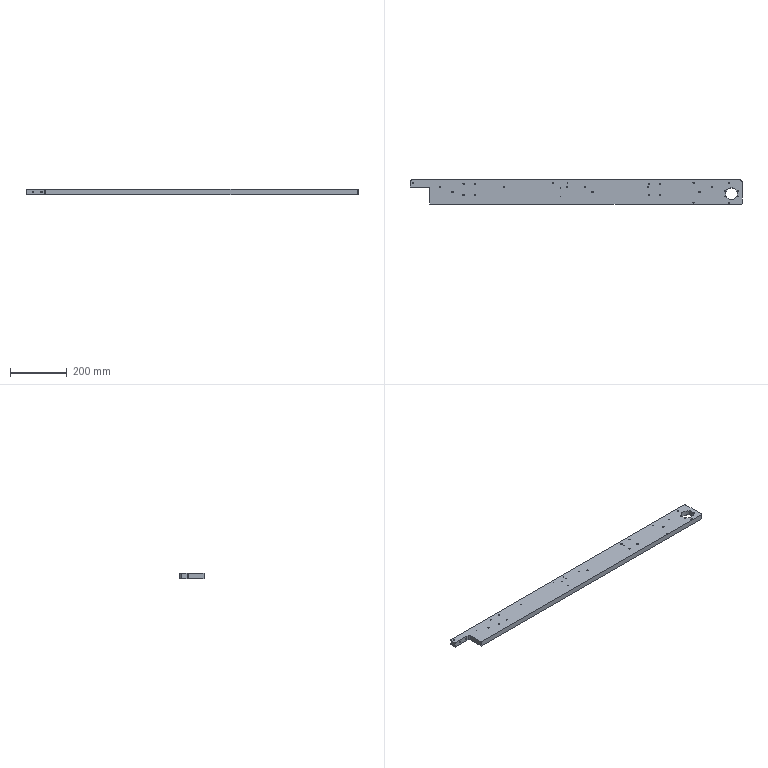Part | STEP file | 1 solid | 149 faces | box 1175 x 85 x 19 mm | volume 1776717 mm3 | cylinder 99 | cone 28 | plane 22 | commonest cylinder face diameters 3.3 x42 5 x16 11 x11 4.2 x8 6 x6 10 x6